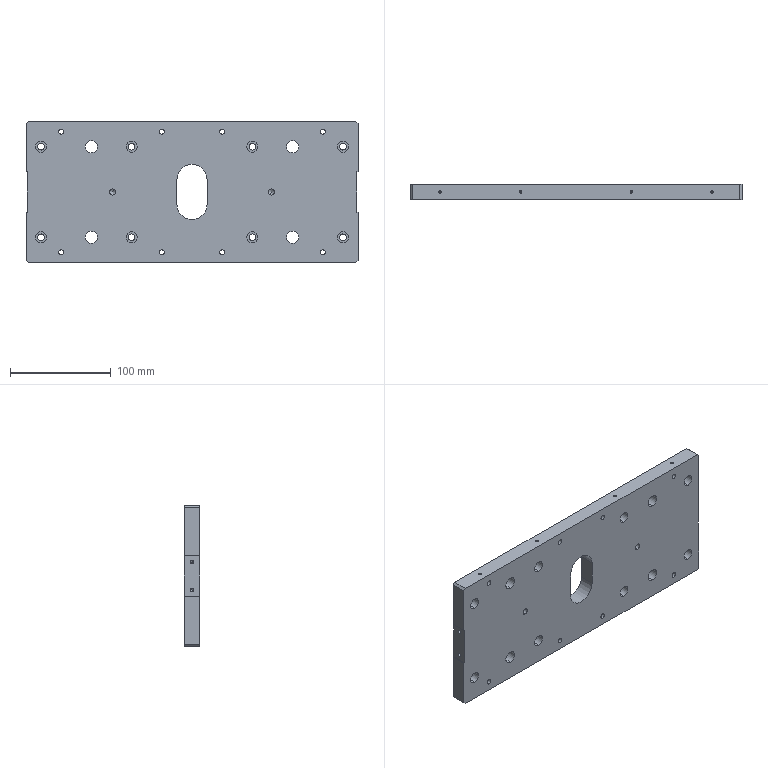Part | SolidWorks | features BaseBody 1 | 1 solid | 167 faces | box 330 x 15 x 140 mm | volume 647095 mm3 | cylinder 103 | plane 36 | cone 28 | commonest cylinder face diameters 2.5 x16 5 x16 6.6 x16 11 x16 20 x16 3.3 x8